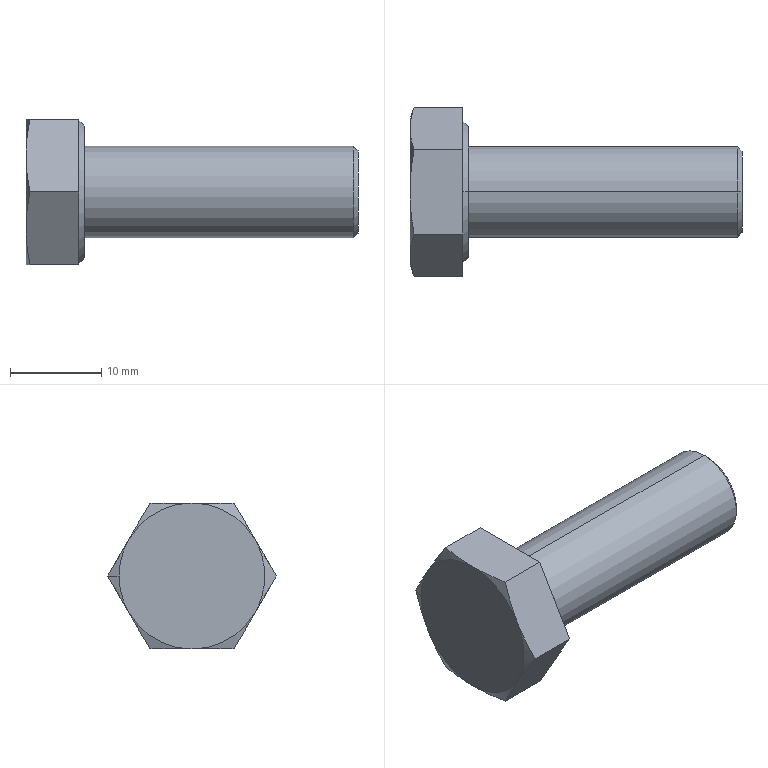Part | STEP file | hex head bolts-full thread grade c gb_GB_FASTENER_BOLT_HHBFTC M10X30-S | 1 solid | 23 faces | box 36.4 x 18.475 x 16 mm | volume 3743 mm3 | cone 11 | plane 10 | cylinder 2 | commonest cylinder face diameters 10 x2
STEP:
#1=CARTESIAN_POINT('',(35.9,0.,5.));
#2=VERTEX_POINT('',#1);
#3=CARTESIAN_POINT('',(35.9,0.,-5.));
#4=VERTEX_POINT('',#3);
#5=CARTESIAN_POINT('',(35.9,0.,0.));
#6=DIRECTION('',(-1.,0.,0.));
#7=DIRECTION('',(0.,0.,1.));
#8=AXIS2_PLACEMENT_3D('',#5,#6,#7);
#9=CIRCLE('',#8,5.);
#10=EDGE_CURVE('',#2,#4,#9,.T.);
#11=ORIENTED_EDGE('',*,*,#10,.T.);
#12=CARTESIAN_POINT('',(6.4,0.,-5.));
#13=VERTEX_POINT('',#12);
#14=CARTESIAN_POINT('',(36.4,0.,-5.));
#15=DIRECTION('',(-1.,0.,0.));
#16=VECTOR('',#15,1000.);
#17=LINE('',#14,#16);
#18=EDGE_CURVE('',#4,#13,#17,.T.);
#19=ORIENTED_EDGE('',*,*,#18,.T.);
#20=CARTESIAN_POINT('',(6.4,0.,5.));
#21=VERTEX_POINT('',#20);
#22=CARTESIAN_POINT('',(6.4,0.,0.));
#23=DIRECTION('',(1.,0.,0.));
#24=DIRECTION('',(0.,0.,1.));
#25=AXIS2_PLACEMENT_3D('',#22,#23,#24);
#26=CIRCLE('',#25,5.);
#27=EDGE_CURVE('',#13,#21,#26,.T.);
#28=ORIENTED_EDGE('',*,*,#27,.T.);
#29=CARTESIAN_POINT('',(36.4,0.,5.));
#30=DIRECTION('',(-1.,0.,0.));
#31=VECTOR('',#30,1000.);
#32=LINE('',#29,#31);
#33=EDGE_CURVE('',#2,#21,#32,.T.);
#34=ORIENTED_EDGE('',*,*,#33,.F.);
#35=EDGE_LOOP('',(#11,#19,#28,#34));
#36=FACE_OUTER_BOUND('',#35,.T.);
#37=CARTESIAN_POINT('',(36.4,0.,0.));
#38=DIRECTION('',(-1.,0.,0.));
#39=DIRECTION('',(0.,0.,1.));
#40=AXIS2_PLACEMENT_3D('',#37,#38,#39);
#41=CYLINDRICAL_SURFACE('',#40,5.);
#42=ADVANCED_FACE('',(#36),#41,.T.);
#43=CARTESIAN_POINT('',(36.4,0.,4.5));
#44=VERTEX_POINT('',#43);
#45=CARTESIAN_POINT('',(36.4,0.,-4.5));
#46=VERTEX_POINT('',#45);
#47=CARTESIAN_POINT('',(36.4,0.,0.));
#48=DIRECTION('',(-1.,0.,0.));
#49=DIRECTION('',(0.,0.,1.));
#50=AXIS2_PLACEMENT_3D('',#47,#48,#49);
#51=CIRCLE('',#50,4.5);
#52=EDGE_CURVE('',#44,#46,#51,.T.);
#53=ORIENTED_EDGE('',*,*,#52,.T.);
#54=CARTESIAN_POINT('',(35.9,0.,-5.));
#55=DIRECTION('',(-0.7071,0.,-0.7071));
#56=VECTOR('',#55,1000.);
#57=LINE('',#54,#56);
#58=EDGE_CURVE('',#46,#4,#57,.T.);
#59=ORIENTED_EDGE('',*,*,#58,.T.);
#60=ORIENTED_EDGE('',*,*,#10,.F.);
#61=CARTESIAN_POINT('',(35.9,0.,5.));
#62=DIRECTION('',(-0.7071,0.,0.7071));
#63=VECTOR('',#62,1000.);
#64=LINE('',#61,#63);
#65=EDGE_CURVE('',#44,#2,#64,.T.);
#66=ORIENTED_EDGE('',*,*,#65,.F.);
#67=EDGE_LOOP('',(#53,#59,#60,#66));
#68=FACE_OUTER_BOUND('',#67,.T.);
#69=CARTESIAN_POINT('',(35.9,0.,0.));
#70=DIRECTION('',(-1.,0.,0.));
#71=DIRECTION('',(0.,0.,1.));
#72=AXIS2_PLACEMENT_3D('',#69,#70,#71);
#73=CONICAL_SURFACE('',#72,5.,0.7854);
#74=ADVANCED_FACE('',(#68),#73,.T.);
#75=CARTESIAN_POINT('',(6.4,0.,7.235));
#76=VERTEX_POINT('',#75);
#77=CARTESIAN_POINT('',(6.4,0.,-7.235));
#78=VERTEX_POINT('',#77);
#79=CARTESIAN_POINT('',(6.4,0.,0.));
#80=DIRECTION('',(-1.,0.,0.));
#81=DIRECTION('',(0.,0.,1.));
#82=AXIS2_PLACEMENT_3D('',#79,#80,#81);
#83=CIRCLE('',#82,7.235);
#84=EDGE_CURVE('',#76,#78,#83,.T.);
#85=ORIENTED_EDGE('',*,*,#84,.T.);
#86=CARTESIAN_POINT('',(5.8,0.,-7.835));
#87=VERTEX_POINT('',#86);
#88=CARTESIAN_POINT('',(5.8,0.,-7.835));
#89=DIRECTION('',(-0.7071,0.,-0.7071));
#90=VECTOR('',#89,1000.);
#91=LINE('',#88,#90);
#92=EDGE_CURVE('',#78,#87,#91,.T.);
#93=ORIENTED_EDGE('',*,*,#92,.T.);
#94=CARTESIAN_POINT('',(5.8,0.,7.835));
#95=VERTEX_POINT('',#94);
#96=CARTESIAN_POINT('',(5.8,0.,0.));
#97=DIRECTION('',(1.,0.,0.));
#98=DIRECTION('',(0.,0.,1.));
#99=AXIS2_PLACEMENT_3D('',#96,#97,#98);
#100=CIRCLE('',#99,7.835);
#101=EDGE_CURVE('',#87,#95,#100,.T.);
#102=ORIENTED_EDGE('',*,*,#101,.T.);
#103=CARTESIAN_POINT('',(5.8,0.,7.835));
#104=DIRECTION('',(-0.7071,0.,0.7071));
#105=VECTOR('',#104,1000.);
#106=LINE('',#103,#105);
#107=EDGE_CURVE('',#76,#95,#106,.T.);
#108=ORIENTED_EDGE('',*,*,#107,.F.);
#109=EDGE_LOOP('',(#85,#93,#102,#108));
#110=FACE_OUTER_BOUND('',#109,.T.);
#111=CARTESIAN_POINT('',(5.8,0.,0.));
#112=DIRECTION('',(-1.,0.,0.));
#113=DIRECTION('',(0.,0.,1.));
#114=AXIS2_PLACEMENT_3D('',#111,#112,#113);
#115=CONICAL_SURFACE('',#114,7.835,0.7854);
#116=ADVANCED_FACE('',(#110),#115,.T.);
#117=CARTESIAN_POINT('',(0.,6.928,-4.));
#118=VERTEX_POINT('',#117);
#119=CARTESIAN_POINT('',(0.,8.,0.));
#120=VERTEX_POINT('',#119);
#121=CARTESIAN_POINT('',(0.,0.,0.));
#122=DIRECTION('',(1.,0.,0.));
#123=DIRECTION('',(0.,1.,0.));
#124=AXIS2_PLACEMENT_3D('',#121,#122,#123);
#125=CIRCLE('',#124,8.);
#126=EDGE_CURVE('',#118,#120,#125,.T.);
#127=ORIENTED_EDGE('',*,*,#126,.T.);
#128=CARTESIAN_POINT('',(0.4505,9.238,0.));
#129=VERTEX_POINT('',#128);
#130=CARTESIAN_POINT('',(0.4532,9.245,0.));
#131=DIRECTION('',(0.342,0.9397,0.));
#132=VECTOR('',#131,1000.);
#133=LINE('',#130,#132);
#134=EDGE_CURVE('',#120,#129,#133,.T.);
#135=ORIENTED_EDGE('',*,*,#134,.T.);
#136=CARTESIAN_POINT('',(0.4505,9.238,0.));
#137=CARTESIAN_POINT('',(0.3115,8.856,-0.6613));
#138=CARTESIAN_POINT('',(0.1979,8.473,-1.325));
#139=CARTESIAN_POINT('',(0.04194,7.703,-2.658));
#140=CARTESIAN_POINT('',(0.,7.317,-3.327));
#141=CARTESIAN_POINT('',(0.,6.928,-4.));
#142=B_SPLINE_CURVE_WITH_KNOTS('',3,(#136,#137,#138,#139,#140,#141),.UNSPECIFIED.,.F.,.F.,(4,2,4),(0.,0.00232,0.004641),.UNSPECIFIED.);
#143=EDGE_CURVE('',#129,#118,#142,.T.);
#144=ORIENTED_EDGE('',*,*,#143,.T.);
#145=EDGE_LOOP('',(#127,#135,#144));
#146=FACE_OUTER_BOUND('',#145,.T.);
#147=CARTESIAN_POINT('',(0.4532,0.,0.));
#148=DIRECTION('',(1.,0.,0.));
#149=DIRECTION('',(0.,1.,0.));
#150=AXIS2_PLACEMENT_3D('',#147,#148,#149);
#151=CONICAL_SURFACE('',#150,9.245,1.222);
#152=ADVANCED_FACE('',(#146),#151,.T.);
#153=ORIENTED_EDGE('',*,*,#18,.F.);
#154=CARTESIAN_POINT('',(35.9,0.,0.));
#155=DIRECTION('',(-1.,0.,0.));
#156=DIRECTION('',(0.,0.,1.));
#157=AXIS2_PLACEMENT_3D('',#154,#155,#156);
#158=CIRCLE('',#157,5.);
#159=EDGE_CURVE('',#4,#2,#158,.T.);
#160=ORIENTED_EDGE('',*,*,#159,.T.);
#161=ORIENTED_EDGE('',*,*,#33,.T.);
#162=CARTESIAN_POINT('',(6.4,0.,0.));
#163=DIRECTION('',(1.,0.,0.));
#164=DIRECTION('',(0.,0.,1.));
#165=AXIS2_PLACEMENT_3D('',#162,#163,#164);
#166=CIRCLE('',#165,5.);
#167=EDGE_CURVE('',#21,#13,#166,.T.);
#168=ORIENTED_EDGE('',*,*,#167,.T.);
#169=EDGE_LOOP('',(#153,#160,#161,#168));
#170=FACE_OUTER_BOUND('',#169,.T.);
#171=CARTESIAN_POINT('',(36.4,0.,0.));
#172=DIRECTION('',(-1.,0.,0.));
#173=DIRECTION('',(0.,0.,1.));
#174=AXIS2_PLACEMENT_3D('',#171,#172,#173);
#175=CYLINDRICAL_SURFACE('',#174,5.);
#176=ADVANCED_FACE('',(#170),#175,.T.);
#177=ORIENTED_EDGE('',*,*,#167,.F.);
#178=ORIENTED_EDGE('',*,*,#27,.F.);
#179=EDGE_LOOP('',(#177,#178));
#180=FACE_BOUND('',#179,.T.);
#181=ORIENTED_EDGE('',*,*,#84,.F.);
#182=CARTESIAN_POINT('',(6.4,0.,0.));
#183=DIRECTION('',(-1.,0.,0.));
#184=DIRECTION('',(0.,0.,1.));
#185=AXIS2_PLACEMENT_3D('',#182,#183,#184);
#186=CIRCLE('',#185,7.235);
#187=EDGE_CURVE('',#78,#76,#186,.T.);
#188=ORIENTED_EDGE('',*,*,#187,.F.);
#189=EDGE_LOOP('',(#181,#188));
#190=FACE_OUTER_BOUND('',#189,.T.);
#191=CARTESIAN_POINT('',(6.4,0.,16.));
#192=DIRECTION('',(-1.,0.,0.));
#193=DIRECTION('',(0.,0.,1.));
#194=AXIS2_PLACEMENT_3D('',#191,#192,#193);
#195=PLANE('',#194);
#196=ADVANCED_FACE('',(#180,#190),#195,.F.);
#197=ORIENTED_EDGE('',*,*,#58,.F.);
#198=CARTESIAN_POINT('',(36.4,0.,0.));
#199=DIRECTION('',(-1.,0.,0.));
#200=DIRECTION('',(0.,0.,1.));
#201=AXIS2_PLACEMENT_3D('',#198,#199,#200);
#202=CIRCLE('',#201,4.5);
#203=EDGE_CURVE('',#46,#44,#202,.T.);
#204=ORIENTED_EDGE('',*,*,#203,.T.);
#205=ORIENTED_EDGE('',*,*,#65,.T.);
#206=ORIENTED_EDGE('',*,*,#159,.F.);
#207=EDGE_LOOP('',(#197,#204,#205,#206));
#208=FACE_OUTER_BOUND('',#207,.T.);
#209=CARTESIAN_POINT('',(35.9,0.,0.));
#210=DIRECTION('',(-1.,0.,0.));
#211=DIRECTION('',(0.,0.,1.));
#212=AXIS2_PLACEMENT_3D('',#209,#210,#211);
#213=CONICAL_SURFACE('',#212,5.,0.7854);
#214=ADVANCED_FACE('',(#208),#213,.T.);
#215=ORIENTED_EDGE('',*,*,#92,.F.);
#216=ORIENTED_EDGE('',*,*,#187,.T.);
#217=ORIENTED_EDGE('',*,*,#107,.T.);
#218=CARTESIAN_POINT('',(5.8,0.,0.));
#219=DIRECTION('',(1.,0.,0.));
#220=DIRECTION('',(0.,0.,1.));
#221=AXIS2_PLACEMENT_3D('',#218,#219,#220);
#222=CIRCLE('',#221,7.835);
#223=EDGE_CURVE('',#95,#87,#222,.T.);
#224=ORIENTED_EDGE('',*,*,#223,.T.);
#225=EDGE_LOOP('',(#215,#216,#217,#224));
#226=FACE_OUTER_BOUND('',#225,.T.);
#227=CARTESIAN_POINT('',(5.8,0.,0.));
#228=DIRECTION('',(-1.,0.,0.));
#229=DIRECTION('',(0.,0.,1.));
#230=AXIS2_PLACEMENT_3D('',#227,#228,#229);
#231=CONICAL_SURFACE('',#230,7.835,0.7854);
#232=ADVANCED_FACE('',(#226),#231,.T.);
#233=ORIENTED_EDGE('',*,*,#52,.F.);
#234=ORIENTED_EDGE('',*,*,#203,.F.);
#235=EDGE_LOOP('',(#233,#234));
#236=FACE_OUTER_BOUND('',#235,.T.);
#237=CARTESIAN_POINT('',(36.4,0.,0.));
#238=DIRECTION('',(1.,0.,0.));
#239=DIRECTION('',(0.,0.,-1.));
#240=AXIS2_PLACEMENT_3D('',#237,#238,#239);
#241=PLANE('',#240);
#242=ADVANCED_FACE('',(#236),#241,.T.);
#243=CARTESIAN_POINT('',(5.8,9.238,0.));
#244=VERTEX_POINT('',#243);
#245=CARTESIAN_POINT('',(5.8,4.619,8.));
#246=VERTEX_POINT('',#245);
#247=CARTESIAN_POINT('',(5.8,9.238,0.));
#248=DIRECTION('',(0.,-0.5,0.866));
#249=VECTOR('',#248,1000.);
#250=LINE('',#247,#249);
#251=EDGE_CURVE('',#244,#246,#250,.T.);
#252=ORIENTED_EDGE('',*,*,#251,.T.);
#253=CARTESIAN_POINT('',(5.8,-4.619,8.));
#254=VERTEX_POINT('',#253);
#255=CARTESIAN_POINT('',(5.8,7.835,8.));
#256=DIRECTION('',(0.,-1.,0.));
#257=VECTOR('',#256,1000.);
#258=LINE('',#255,#257);
#259=EDGE_CURVE('',#246,#254,#258,.T.);
#260=ORIENTED_EDGE('',*,*,#259,.T.);
#261=CARTESIAN_POINT('',(5.8,-9.238,0.));
#262=VERTEX_POINT('',#261);
#263=CARTESIAN_POINT('',(5.8,-4.619,8.));
#264=DIRECTION('',(0.,-0.5,-0.866));
#265=VECTOR('',#264,1000.);
#266=LINE('',#263,#265);
#267=EDGE_CURVE('',#254,#262,#266,.T.);
#268=ORIENTED_EDGE('',*,*,#267,.T.);
#269=CARTESIAN_POINT('',(5.8,-4.619,-8.));
#270=VERTEX_POINT('',#269);
#271=CARTESIAN_POINT('',(5.8,-9.238,0.));
#272=DIRECTION('',(0.,0.5,-0.866));
#273=VECTOR('',#272,1000.);
#274=LINE('',#271,#273);
#275=EDGE_CURVE('',#262,#270,#274,.T.);
#276=ORIENTED_EDGE('',*,*,#275,.T.);
#277=CARTESIAN_POINT('',(5.8,4.619,-8.));
#278=VERTEX_POINT('',#277);
#279=CARTESIAN_POINT('',(5.8,7.835,-8.));
#280=DIRECTION('',(0.,1.,0.));
#281=VECTOR('',#280,1000.);
#282=LINE('',#279,#281);
#283=EDGE_CURVE('',#270,#278,#282,.T.);
#284=ORIENTED_EDGE('',*,*,#283,.T.);
#285=CARTESIAN_POINT('',(5.8,4.619,-8.));
#286=DIRECTION('',(0.,0.5,0.866));
#287=VECTOR('',#286,1000.);
#288=LINE('',#285,#287);
#289=EDGE_CURVE('',#278,#244,#288,.T.);
#290=ORIENTED_EDGE('',*,*,#289,.T.);
#291=EDGE_LOOP('',(#252,#260,#268,#276,#284,#290));
#292=FACE_OUTER_BOUND('',#291,.T.);
#293=ORIENTED_EDGE('',*,*,#223,.F.);
#294=ORIENTED_EDGE('',*,*,#101,.F.);
#295=EDGE_LOOP('',(#293,#294));
#296=FACE_BOUND('',#295,.T.);
#297=CARTESIAN_POINT('',(5.8,7.835,0.));
#298=DIRECTION('',(1.,0.,0.));
#299=DIRECTION('',(0.,0.,-1.));
#300=AXIS2_PLACEMENT_3D('',#297,#298,#299);
#301=PLANE('',#300);
#302=ADVANCED_FACE('',(#292,#296),#301,.T.);
#303=CARTESIAN_POINT('',(0.4505,-4.619,8.));
#304=VERTEX_POINT('',#303);
#305=CARTESIAN_POINT('',(6.4,-4.619,8.));
#306=DIRECTION('',(-1.,0.,0.));
#307=VECTOR('',#306,1000.);
#308=LINE('',#305,#307);
#309=EDGE_CURVE('',#254,#304,#308,.T.);
#310=ORIENTED_EDGE('',*,*,#309,.F.);
#311=ORIENTED_EDGE('',*,*,#259,.F.);
#312=CARTESIAN_POINT('',(0.4505,4.619,8.));
#313=VERTEX_POINT('',#312);
#314=CARTESIAN_POINT('',(6.4,4.619,8.));
#315=DIRECTION('',(1.,0.,0.));
#316=VECTOR('',#315,1000.);
#317=LINE('',#314,#316);
#318=EDGE_CURVE('',#313,#246,#317,.T.);
#319=ORIENTED_EDGE('',*,*,#318,.F.);
#320=CARTESIAN_POINT('',(0.,0.,8.));
#321=VERTEX_POINT('',#320);
#322=CARTESIAN_POINT('',(0.,0.,8.));
#323=CARTESIAN_POINT('',(0.,0.7771,8.));
#324=CARTESIAN_POINT('',(0.04194,1.55,8.));
#325=CARTESIAN_POINT('',(0.1979,3.089,8.));
#326=CARTESIAN_POINT('',(0.3115,3.855,8.));
#327=CARTESIAN_POINT('',(0.4505,4.619,8.));
#328=B_SPLINE_CURVE_WITH_KNOTS('',3,(#322,#323,#324,#325,#326,#327),.UNSPECIFIED.,.F.,.F.,(4,2,4),(0.,0.00232,0.004641),.UNSPECIFIED.);
#329=EDGE_CURVE('',#321,#313,#328,.T.);
#330=ORIENTED_EDGE('',*,*,#329,.F.);
#331=CARTESIAN_POINT('',(0.4505,-4.619,8.));
#332=CARTESIAN_POINT('',(0.3115,-3.855,8.));
#333=CARTESIAN_POINT('',(0.1979,-3.089,8.));
#334=CARTESIAN_POINT('',(0.04194,-1.55,8.));
#335=CARTESIAN_POINT('',(0.,-0.7771,8.));
#336=CARTESIAN_POINT('',(0.,0.,8.));
#337=B_SPLINE_CURVE_WITH_KNOTS('',3,(#331,#332,#333,#334,#335,#336),.UNSPECIFIED.,.F.,.F.,(4,2,4),(0.,0.00232,0.004641),.UNSPECIFIED.);
#338=EDGE_CURVE('',#304,#321,#337,.T.);
#339=ORIENTED_EDGE('',*,*,#338,.F.);
#340=EDGE_LOOP('',(#310,#311,#319,#330,#339));
#341=FACE_OUTER_BOUND('',#340,.T.);
#342=CARTESIAN_POINT('',(6.4,4.619,8.));
#343=DIRECTION('',(0.,0.,-1.));
#344=DIRECTION('',(-1.,0.,0.));
#345=AXIS2_PLACEMENT_3D('',#342,#343,#344);
#346=PLANE('',#345);
#347=ADVANCED_FACE('',(#341),#346,.F.);
#348=ORIENTED_EDGE('',*,*,#318,.T.);
#349=ORIENTED_EDGE('',*,*,#251,.F.);
#350=CARTESIAN_POINT('',(6.4,9.238,0.));
#351=DIRECTION('',(1.,0.,0.));
#352=VECTOR('',#351,1000.);
#353=LINE('',#350,#352);
#354=EDGE_CURVE('',#129,#244,#353,.T.);
#355=ORIENTED_EDGE('',*,*,#354,.F.);
#356=CARTESIAN_POINT('',(0.,6.928,4.));
#357=VERTEX_POINT('',#356);
#358=CARTESIAN_POINT('',(0.,6.928,4.));
#359=CARTESIAN_POINT('',(0.,7.317,3.327));
#360=CARTESIAN_POINT('',(0.04194,7.703,2.658));
#361=CARTESIAN_POINT('',(0.1979,8.473,1.325));
#362=CARTESIAN_POINT('',(0.3115,8.856,0.6613));
#363=CARTESIAN_POINT('',(0.4505,9.238,0.));
#364=B_SPLINE_CURVE_WITH_KNOTS('',3,(#358,#359,#360,#361,#362,#363),.UNSPECIFIED.,.F.,.F.,(4,2,4),(0.,0.00232,0.004641),.UNSPECIFIED.);
#365=EDGE_CURVE('',#357,#129,#364,.T.);
#366=ORIENTED_EDGE('',*,*,#365,.F.);
#367=CARTESIAN_POINT('',(0.4505,4.619,8.));
#368=CARTESIAN_POINT('',(0.3115,5.001,7.339));
#369=CARTESIAN_POINT('',(0.1979,5.384,6.675));
#370=CARTESIAN_POINT('',(0.04194,6.153,5.342));
#371=CARTESIAN_POINT('',(0.,6.54,4.673));
#372=CARTESIAN_POINT('',(0.,6.928,4.));
#373=B_SPLINE_CURVE_WITH_KNOTS('',3,(#367,#368,#369,#370,#371,#372),.UNSPECIFIED.,.F.,.F.,(4,2,4),(0.,0.00232,0.004641),.UNSPECIFIED.);
#374=EDGE_CURVE('',#313,#357,#373,.T.);
#375=ORIENTED_EDGE('',*,*,#374,.F.);
#376=EDGE_LOOP('',(#348,#349,#355,#366,#375));
#377=FACE_OUTER_BOUND('',#376,.T.);
#378=CARTESIAN_POINT('',(6.4,9.238,0.));
#379=DIRECTION('',(0.,-0.866,-0.5));
#380=DIRECTION('',(0.,0.5,-0.866));
#381=AXIS2_PLACEMENT_3D('',#378,#379,#380);
#382=PLANE('',#381);
#383=ADVANCED_FACE('',(#377),#382,.F.);
#384=ORIENTED_EDGE('',*,*,#354,.T.);
#385=ORIENTED_EDGE('',*,*,#289,.F.);
#386=CARTESIAN_POINT('',(0.4505,4.619,-8.));
#387=VERTEX_POINT('',#386);
#388=CARTESIAN_POINT('',(6.4,4.619,-8.));
#389=DIRECTION('',(1.,0.,0.));
#390=VECTOR('',#389,1000.);
#391=LINE('',#388,#390);
#392=EDGE_CURVE('',#387,#278,#391,.T.);
#393=ORIENTED_EDGE('',*,*,#392,.F.);
#394=CARTESIAN_POINT('',(0.,6.928,-4.));
#395=CARTESIAN_POINT('',(0.,6.54,-4.673));
#396=CARTESIAN_POINT('',(0.04194,6.153,-5.342));
#397=CARTESIAN_POINT('',(0.1979,5.384,-6.675));
#398=CARTESIAN_POINT('',(0.3115,5.001,-7.339));
#399=CARTESIAN_POINT('',(0.4505,4.619,-8.));
#400=B_SPLINE_CURVE_WITH_KNOTS('',3,(#394,#395,#396,#397,#398,#399),.UNSPECIFIED.,.F.,.F.,(4,2,4),(0.,0.00232,0.004641),.UNSPECIFIED.);
#401=EDGE_CURVE('',#118,#387,#400,.T.);
#402=ORIENTED_EDGE('',*,*,#401,.F.);
#403=ORIENTED_EDGE('',*,*,#143,.F.);
#404=EDGE_LOOP('',(#384,#385,#393,#402,#403));
#405=FACE_OUTER_BOUND('',#404,.T.);
#406=CARTESIAN_POINT('',(6.4,4.619,-8.));
#407=DIRECTION('',(0.,-0.866,0.5));
#408=DIRECTION('',(0.,-0.5,-0.866));
#409=AXIS2_PLACEMENT_3D('',#406,#407,#408);
#410=PLANE('',#409);
#411=ADVANCED_FACE('',(#405),#410,.F.);
#412=ORIENTED_EDGE('',*,*,#392,.T.);
#413=ORIENTED_EDGE('',*,*,#283,.F.);
#414=CARTESIAN_POINT('',(0.4505,-4.619,-8.));
#415=VERTEX_POINT('',#414);
#416=CARTESIAN_POINT('',(6.4,-4.619,-8.));
#417=DIRECTION('',(1.,0.,0.));
#418=VECTOR('',#417,1000.);
#419=LINE('',#416,#418);
#420=EDGE_CURVE('',#415,#270,#419,.T.);
#421=ORIENTED_EDGE('',*,*,#420,.F.);
#422=CARTESIAN_POINT('',(0.,0.,-8.));
#423=VERTEX_POINT('',#422);
#424=CARTESIAN_POINT('',(0.,0.,-8.));
#425=CARTESIAN_POINT('',(0.,-0.7771,-8.));
#426=CARTESIAN_POINT('',(0.04194,-1.55,-8.));
#427=CARTESIAN_POINT('',(0.1979,-3.089,-8.));
#428=CARTESIAN_POINT('',(0.3115,-3.855,-8.));
#429=CARTESIAN_POINT('',(0.4505,-4.619,-8.));
#430=B_SPLINE_CURVE_WITH_KNOTS('',3,(#424,#425,#426,#427,#428,#429),.UNSPECIFIED.,.F.,.F.,(4,2,4),(0.,0.00232,0.004641),.UNSPECIFIED.);
#431=EDGE_CURVE('',#423,#415,#430,.T.);
#432=ORIENTED_EDGE('',*,*,#431,.F.);
#433=CARTESIAN_POINT('',(0.4505,4.619,-8.));
#434=CARTESIAN_POINT('',(0.3115,3.855,-8.));
#435=CARTESIAN_POINT('',(0.1979,3.089,-8.));
#436=CARTESIAN_POINT('',(0.04194,1.55,-8.));
#437=CARTESIAN_POINT('',(0.,0.7771,-8.));
#438=CARTESIAN_POINT('',(0.,0.,-8.));
#439=B_SPLINE_CURVE_WITH_KNOTS('',3,(#433,#434,#435,#436,#437,#438),.UNSPECIFIED.,.F.,.F.,(4,2,4),(0.,0.00232,0.004641),.UNSPECIFIED.);
#440=EDGE_CURVE('',#387,#423,#439,.T.);
#441=ORIENTED_EDGE('',*,*,#440,.F.);
#442=EDGE_LOOP('',(#412,#413,#421,#432,#441));
#443=FACE_OUTER_BOUND('',#442,.T.);
#444=CARTESIAN_POINT('',(6.4,-4.619,-8.));
#445=DIRECTION('',(0.,0.,1.));
#446=DIRECTION('',(0.,-1.,0.));
#447=AXIS2_PLACEMENT_3D('',#444,#445,#446);
#448=PLANE('',#447);
#449=ADVANCED_FACE('',(#443),#448,.F.);
#450=ORIENTED_EDGE('',*,*,#420,.T.);
#451=ORIENTED_EDGE('',*,*,#275,.F.);
#452=CARTESIAN_POINT('',(0.4505,-9.238,0.));
#453=VERTEX_POINT('',#452);
#454=CARTESIAN_POINT('',(6.4,-9.238,0.));
#455=DIRECTION('',(1.,0.,0.));
#456=VECTOR('',#455,1000.);
#457=LINE('',#454,#456);
#458=EDGE_CURVE('',#453,#262,#457,.T.);
#459=ORIENTED_EDGE('',*,*,#458,.F.);
#460=CARTESIAN_POINT('',(0.,-6.928,-4.));
#461=VERTEX_POINT('',#460);
#462=CARTESIAN_POINT('',(0.,-6.928,-4.));
#463=CARTESIAN_POINT('',(0.,-7.317,-3.327));
#464=CARTESIAN_POINT('',(0.04194,-7.703,-2.658));
#465=CARTESIAN_POINT('',(0.1979,-8.473,-1.325));
#466=CARTESIAN_POINT('',(0.3115,-8.856,-0.6613));
#467=CARTESIAN_POINT('',(0.4505,-9.238,0.));
#468=B_SPLINE_CURVE_WITH_KNOTS('',3,(#462,#463,#464,#465,#466,#467),.UNSPECIFIED.,.F.,.F.,(4,2,4),(0.,0.00232,0.004641),.UNSPECIFIED.);
#469=EDGE_CURVE('',#461,#453,#468,.T.);
#470=ORIENTED_EDGE('',*,*,#469,.F.);
#471=CARTESIAN_POINT('',(0.4505,-4.619,-8.));
#472=CARTESIAN_POINT('',(0.3115,-5.001,-7.339));
#473=CARTESIAN_POINT('',(0.1979,-5.384,-6.675));
#474=CARTESIAN_POINT('',(0.04194,-6.153,-5.342));
#475=CARTESIAN_POINT('',(0.,-6.54,-4.673));
#476=CARTESIAN_POINT('',(0.,-6.928,-4.));
#477=B_SPLINE_CURVE_WITH_KNOTS('',3,(#471,#472,#473,#474,#475,#476),.UNSPECIFIED.,.F.,.F.,(4,2,4),(0.,0.00232,0.004641),.UNSPECIFIED.);
#478=EDGE_CURVE('',#415,#461,#477,.T.);
#479=ORIENTED_EDGE('',*,*,#478,.F.);
#480=EDGE_LOOP('',(#450,#451,#459,#470,#479));
#481=FACE_OUTER_BOUND('',#480,.T.);
#482=CARTESIAN_POINT('',(6.4,-9.238,0.));
#483=DIRECTION('',(0.,0.866,0.5));
#484=DIRECTION('',(0.,-0.5,0.866));
#485=AXIS2_PLACEMENT_3D('',#482,#483,#484);
#486=PLANE('',#485);
#487=ADVANCED_FACE('',(#481),#486,.F.);
#488=ORIENTED_EDGE('',*,*,#458,.T.);
#489=ORIENTED_EDGE('',*,*,#267,.F.);
#490=ORIENTED_EDGE('',*,*,#309,.T.);
#491=CARTESIAN_POINT('',(0.,-6.928,4.));
#492=VERTEX_POINT('',#491);
#493=CARTESIAN_POINT('',(0.,-6.928,4.));
#494=CARTESIAN_POINT('',(0.,-6.54,4.673));
#495=CARTESIAN_POINT('',(0.04194,-6.153,5.342));
#496=CARTESIAN_POINT('',(0.1979,-5.384,6.675));
#497=CARTESIAN_POINT('',(0.3115,-5.001,7.339));
#498=CARTESIAN_POINT('',(0.4505,-4.619,8.));
#499=B_SPLINE_CURVE_WITH_KNOTS('',3,(#493,#494,#495,#496,#497,#498),.UNSPECIFIED.,.F.,.F.,(4,2,4),(0.,0.00232,0.004641),.UNSPECIFIED.);
#500=EDGE_CURVE('',#492,#304,#499,.T.);
#501=ORIENTED_EDGE('',*,*,#500,.F.);
#502=CARTESIAN_POINT('',(0.4505,-9.238,0.));
#503=CARTESIAN_POINT('',(0.3115,-8.856,0.6613));
#504=CARTESIAN_POINT('',(0.1979,-8.473,1.325));
#505=CARTESIAN_POINT('',(0.04194,-7.703,2.658));
#506=CARTESIAN_POINT('',(0.,-7.317,3.327));
#507=CARTESIAN_POINT('',(0.,-6.928,4.));
#508=B_SPLINE_CURVE_WITH_KNOTS('',3,(#502,#503,#504,#505,#506,#507),.UNSPECIFIED.,.F.,.F.,(4,2,4),(0.,0.00232,0.004641),.UNSPECIFIED.);
#509=EDGE_CURVE('',#453,#492,#508,.T.);
#510=ORIENTED_EDGE('',*,*,#509,.F.);
#511=EDGE_LOOP('',(#488,#489,#490,#501,#510));
#512=FACE_OUTER_BOUND('',#511,.T.);
#513=CARTESIAN_POINT('',(6.4,-4.619,8.));
#514=DIRECTION('',(0.,0.866,-0.5));
#515=DIRECTION('',(0.,0.5,0.866));
#516=AXIS2_PLACEMENT_3D('',#513,#514,#515);
#517=PLANE('',#516);
#518=ADVANCED_FACE('',(#512),#517,.F.);
#519=ORIENTED_EDGE('',*,*,#338,.T.);
#520=CARTESIAN_POINT('',(0.,0.,0.));
#521=DIRECTION('',(1.,0.,0.));
#522=DIRECTION('',(0.,1.,0.));
#523=AXIS2_PLACEMENT_3D('',#520,#521,#522);
#524=CIRCLE('',#523,8.);
#525=EDGE_CURVE('',#321,#492,#524,.T.);
#526=ORIENTED_EDGE('',*,*,#525,.T.);
#527=ORIENTED_EDGE('',*,*,#500,.T.);
#528=EDGE_LOOP('',(#519,#526,#527));
#529=FACE_OUTER_BOUND('',#528,.T.);
#530=CARTESIAN_POINT('',(0.4532,0.,0.));
#531=DIRECTION('',(1.,0.,0.));
#532=DIRECTION('',(0.,1.,0.));
#533=AXIS2_PLACEMENT_3D('',#530,#531,#532);
#534=CONICAL_SURFACE('',#533,9.245,1.222);
#535=ADVANCED_FACE('',(#529),#534,.T.);
#536=CARTESIAN_POINT('',(0.,0.,0.));
#537=DIRECTION('',(1.,0.,0.));
#538=DIRECTION('',(0.,1.,0.));
#539=AXIS2_PLACEMENT_3D('',#536,#537,#538);
#540=CIRCLE('',#539,8.);
#541=EDGE_CURVE('',#357,#321,#540,.T.);
#542=ORIENTED_EDGE('',*,*,#541,.T.);
#543=ORIENTED_EDGE('',*,*,#329,.T.);
#544=ORIENTED_EDGE('',*,*,#374,.T.);
#545=EDGE_LOOP('',(#542,#543,#544));
#546=FACE_OUTER_BOUND('',#545,.T.);
#547=CARTESIAN_POINT('',(0.4532,0.,0.));
#548=DIRECTION('',(1.,0.,0.));
#549=DIRECTION('',(0.,1.,0.));
#550=AXIS2_PLACEMENT_3D('',#547,#548,#549);
#551=CONICAL_SURFACE('',#550,9.245,1.222);
#552=ADVANCED_FACE('',(#546),#551,.T.);
#553=ORIENTED_EDGE('',*,*,#134,.F.);
#554=CARTESIAN_POINT('',(0.,0.,0.));
#555=DIRECTION('',(1.,0.,0.));
#556=DIRECTION('',(0.,1.,0.));
#557=AXIS2_PLACEMENT_3D('',#554,#555,#556);
#558=CIRCLE('',#557,8.);
#559=EDGE_CURVE('',#120,#357,#558,.T.);
#560=ORIENTED_EDGE('',*,*,#559,.T.);
#561=ORIENTED_EDGE('',*,*,#365,.T.);
#562=EDGE_LOOP('',(#553,#560,#561));
#563=FACE_OUTER_BOUND('',#562,.T.);
#564=CARTESIAN_POINT('',(0.4532,0.,0.));
#565=DIRECTION('',(1.,0.,0.));
#566=DIRECTION('',(0.,1.,0.));
#567=AXIS2_PLACEMENT_3D('',#564,#565,#566);
#568=CONICAL_SURFACE('',#567,9.245,1.222);
#569=ADVANCED_FACE('',(#563),#568,.T.);
#570=CARTESIAN_POINT('',(0.,0.,0.));
#571=DIRECTION('',(1.,0.,0.));
#572=DIRECTION('',(0.,1.,0.));
#573=AXIS2_PLACEMENT_3D('',#570,#571,#572);
#574=CIRCLE('',#573,8.);
#575=EDGE_CURVE('',#423,#118,#574,.T.);
#576=ORIENTED_EDGE('',*,*,#575,.T.);
#577=ORIENTED_EDGE('',*,*,#401,.T.);
#578=ORIENTED_EDGE('',*,*,#440,.T.);
#579=EDGE_LOOP('',(#576,#577,#578));
#580=FACE_OUTER_BOUND('',#579,.T.);
#581=CARTESIAN_POINT('',(0.4532,0.,0.));
#582=DIRECTION('',(1.,0.,0.));
#583=DIRECTION('',(0.,1.,0.));
#584=AXIS2_PLACEMENT_3D('',#581,#582,#583);
#585=CONICAL_SURFACE('',#584,9.245,1.222);
#586=ADVANCED_FACE('',(#580),#585,.T.);
#587=ORIENTED_EDGE('',*,*,#478,.T.);
#588=CARTESIAN_POINT('',(0.,0.,0.));
#589=DIRECTION('',(1.,0.,0.));
#590=DIRECTION('',(0.,1.,0.));
#591=AXIS2_PLACEMENT_3D('',#588,#589,#590);
#592=CIRCLE('',#591,8.);
#593=EDGE_CURVE('',#461,#423,#592,.T.);
#594=ORIENTED_EDGE('',*,*,#593,.T.);
#595=ORIENTED_EDGE('',*,*,#431,.T.);
#596=EDGE_LOOP('',(#587,#594,#595));
#597=FACE_OUTER_BOUND('',#596,.T.);
#598=CARTESIAN_POINT('',(0.4532,0.,0.));
#599=DIRECTION('',(1.,0.,0.));
#600=DIRECTION('',(0.,1.,0.));
#601=AXIS2_PLACEMENT_3D('',#598,#599,#600);
#602=CONICAL_SURFACE('',#601,9.245,1.222);
#603=ADVANCED_FACE('',(#597),#602,.T.);
#604=ORIENTED_EDGE('',*,*,#509,.T.);
#605=CARTESIAN_POINT('',(0.,0.,0.));
#606=DIRECTION('',(1.,0.,0.));
#607=DIRECTION('',(0.,1.,0.));
#608=AXIS2_PLACEMENT_3D('',#605,#606,#607);
#609=CIRCLE('',#608,8.);
#610=EDGE_CURVE('',#492,#461,#609,.T.);
#611=ORIENTED_EDGE('',*,*,#610,.T.);
#612=ORIENTED_EDGE('',*,*,#469,.T.);
#613=EDGE_LOOP('',(#604,#611,#612));
#614=FACE_OUTER_BOUND('',#613,.T.);
#615=CARTESIAN_POINT('',(0.4532,0.,0.));
#616=DIRECTION('',(1.,0.,0.));
#617=DIRECTION('',(0.,1.,0.));
#618=AXIS2_PLACEMENT_3D('',#615,#616,#617);
#619=CONICAL_SURFACE('',#618,9.245,1.222);
#620=ADVANCED_FACE('',(#614),#619,.T.);
#621=ORIENTED_EDGE('',*,*,#593,.F.);
#622=ORIENTED_EDGE('',*,*,#610,.F.);
#623=ORIENTED_EDGE('',*,*,#525,.F.);
#624=ORIENTED_EDGE('',*,*,#541,.F.);
#625=ORIENTED_EDGE('',*,*,#559,.F.);
#626=ORIENTED_EDGE('',*,*,#126,.F.);
#627=ORIENTED_EDGE('',*,*,#575,.F.);
#628=EDGE_LOOP('',(#621,#622,#623,#624,#625,#626,#627));
#629=FACE_OUTER_BOUND('',#628,.T.);
#630=CARTESIAN_POINT('',(0.,0.,16.));
#631=DIRECTION('',(-1.,0.,0.));
#632=DIRECTION('',(0.,0.,1.));
#633=AXIS2_PLACEMENT_3D('',#630,#631,#632);
#634=PLANE('',#633);
#635=ADVANCED_FACE('',(#629),#634,.T.);
#636=CLOSED_SHELL('',(#42,#74,#116,#152,#176,#196,#214,#232,#242,#302,#347,#383,#411,#449,#487,#518,#535,#552,#569,#586,#603,#620,#635));
#637=MANIFOLD_SOLID_BREP('',#636);
#638=CARTESIAN_POINT('',(0.,0.,0.));
#639=DIRECTION('',(0.,0.,1.));
#640=DIRECTION('',(1.,0.,0.));
#641=AXIS2_PLACEMENT_3D('',#638,#639,#640);
#642=(LENGTH_UNIT()NAMED_UNIT(*)SI_UNIT(.MILLI.,.METRE.));
#643=UNCERTAINTY_MEASURE_WITH_UNIT(LENGTH_MEASURE(0.00001),#642,'','');
#644=(NAMED_UNIT(*)PLANE_ANGLE_UNIT()SI_UNIT($,.RADIAN.));
#645=(NAMED_UNIT(*)SI_UNIT($,.STERADIAN.)SOLID_ANGLE_UNIT());
#646=(GEOMETRIC_REPRESENTATION_CONTEXT(3)GLOBAL_UNCERTAINTY_ASSIGNED_CONTEXT((#643))GLOBAL_UNIT_ASSIGNED_CONTEXT((#642,#644,#645))REPRESENTATION_CONTEXT('',''));
#647=ADVANCED_BREP_SHAPE_REPRESENTATION('',(#637,#641),#646);